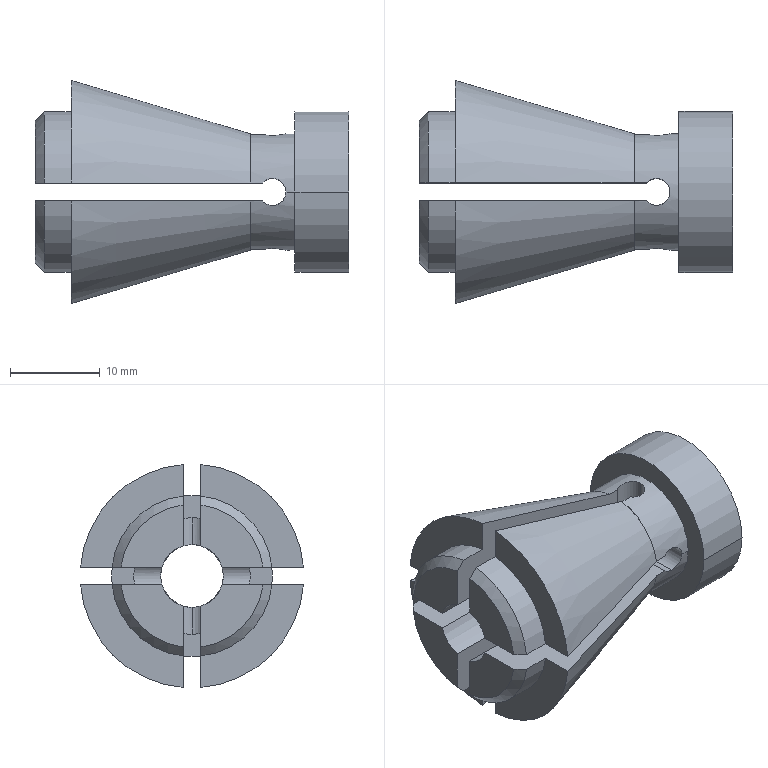Part | SolidWorks | features ICE 5, Chamfer 1, Revolution 1 | 1 solid | 50 faces | box 35 x 24.92 x 24.92 mm | volume 6477 mm3 | plane 22 | cylinder 20 | cone 8 | commonest cylinder face diameters 3 x10 18 x6 7 x2 13 x2